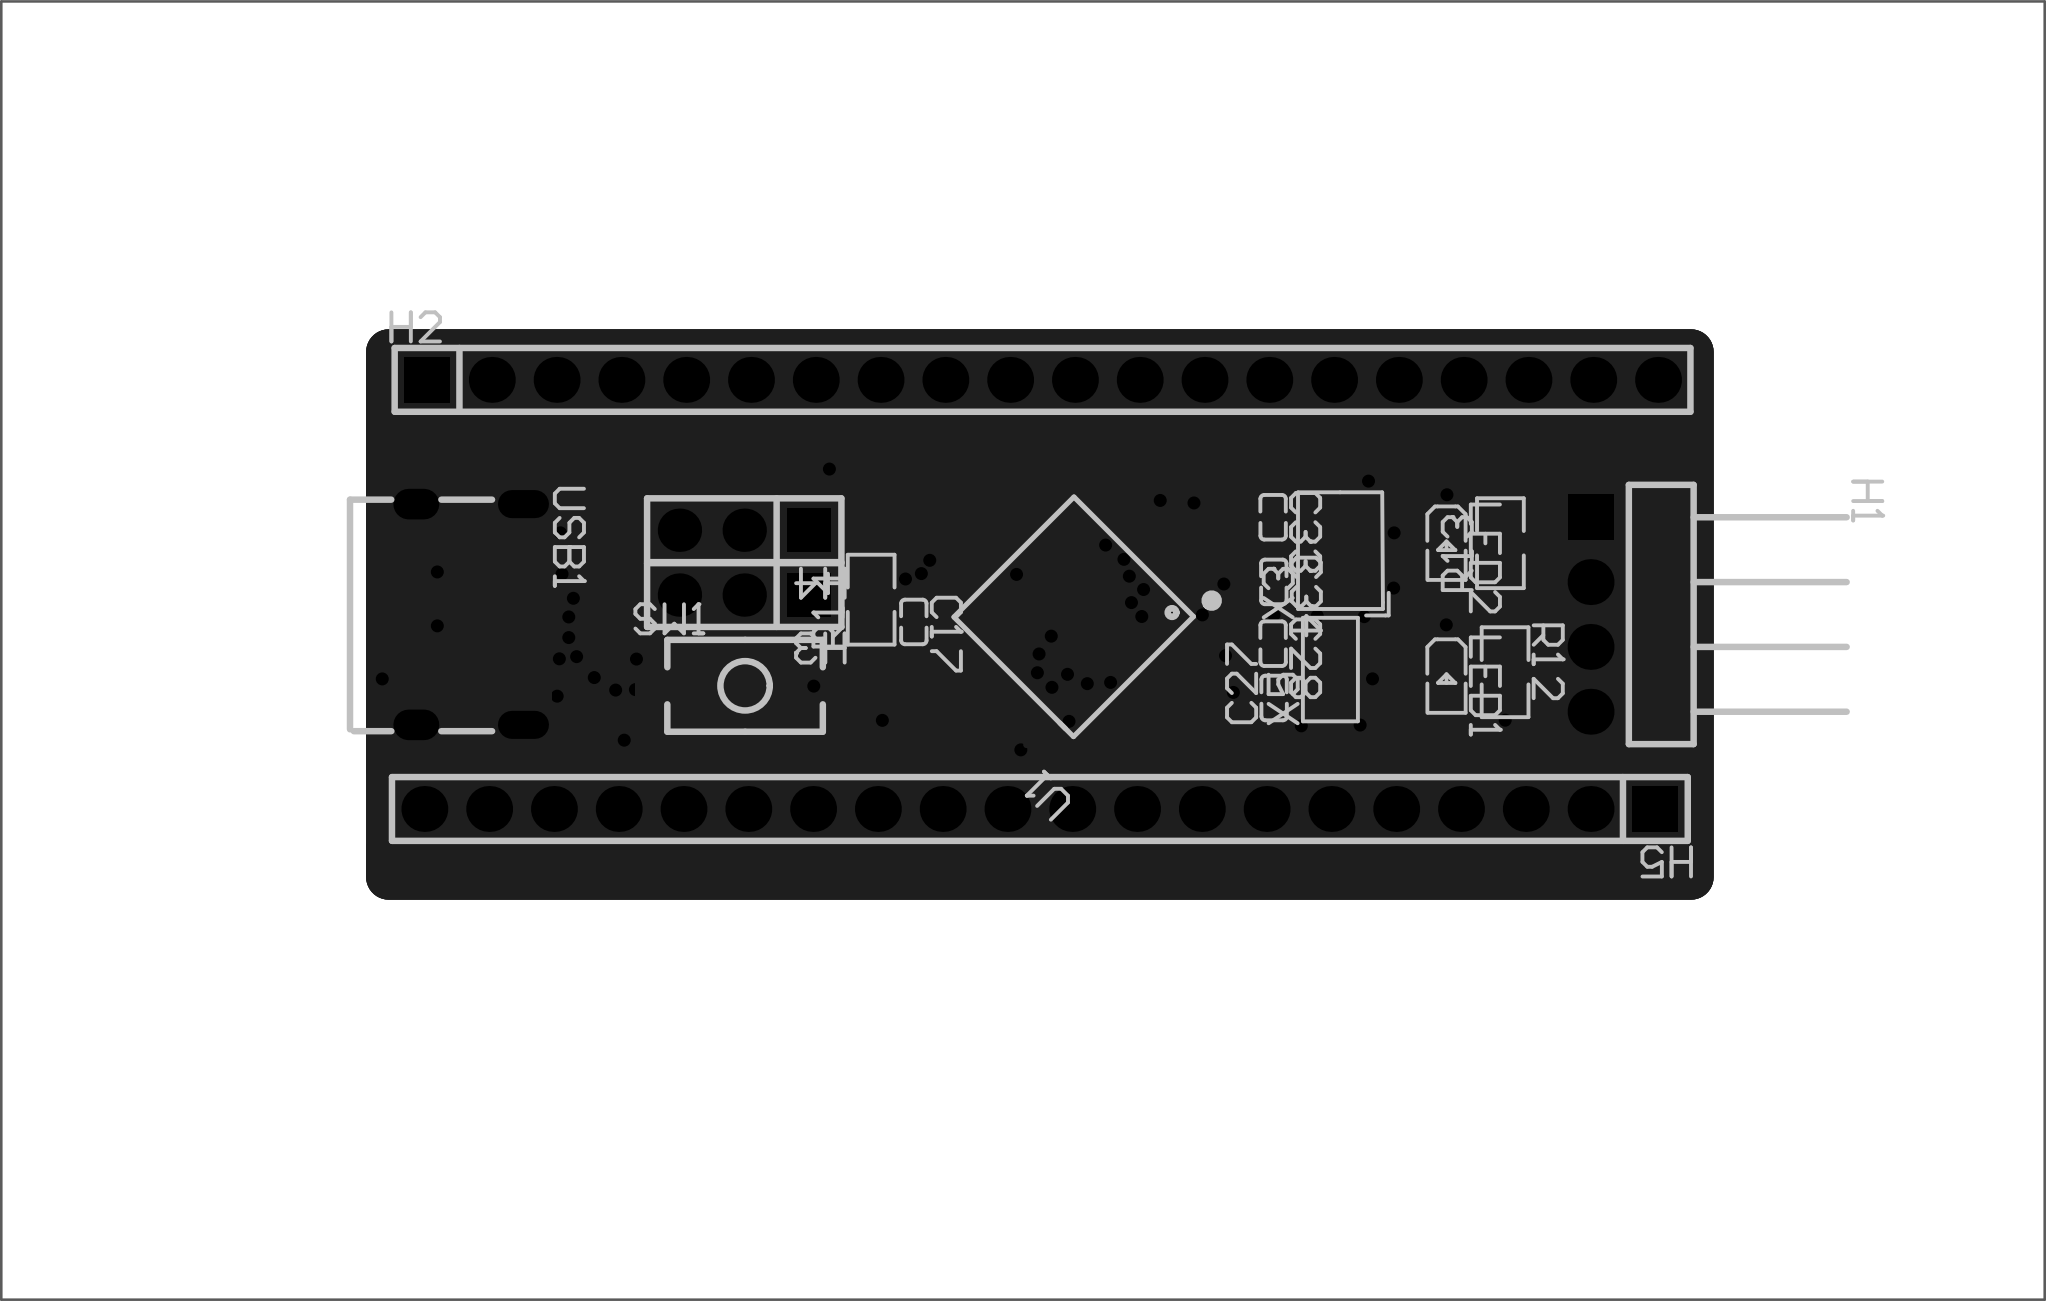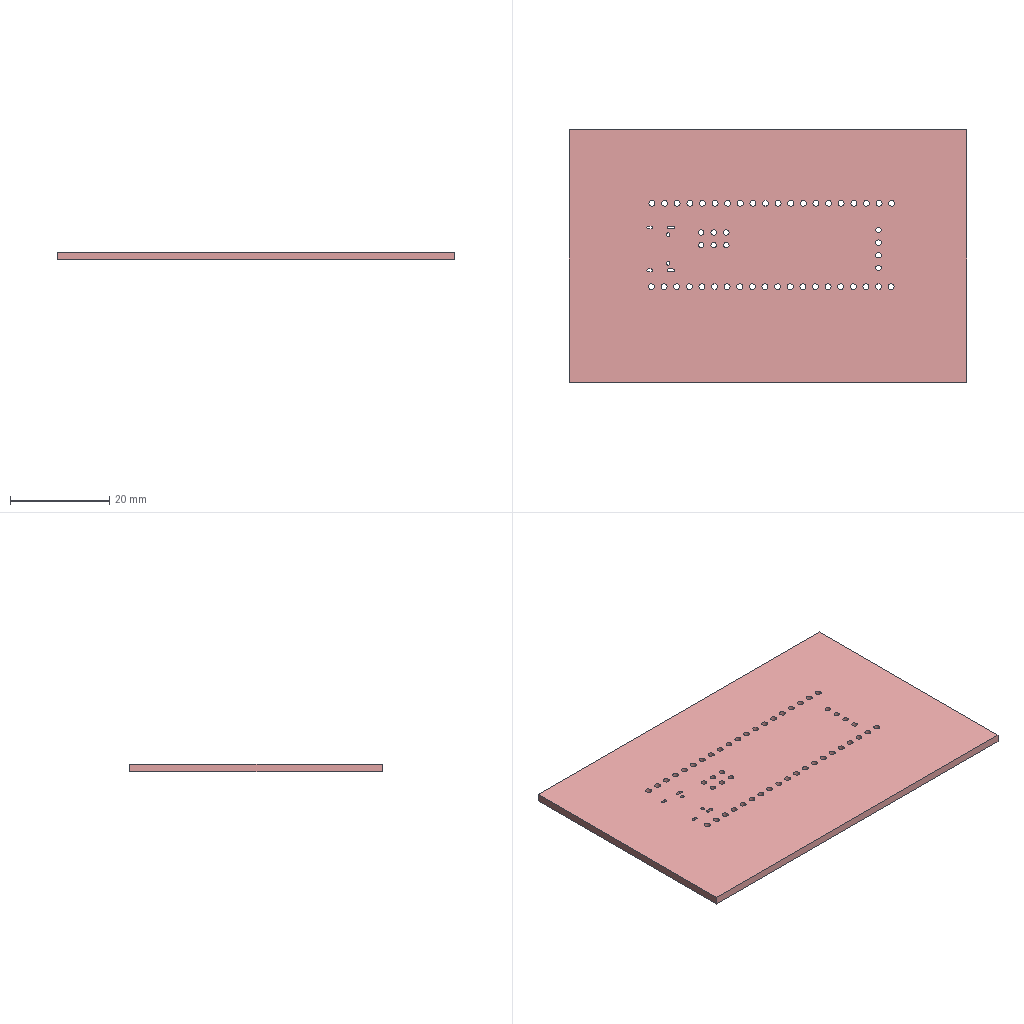Circuit board layout | Altium Designer | box 80.1 x 50.9 x 1.6 mm
Layer stack:
# Altium Designer layer stack of  (unit mm; dielectric type: 0 none, 1 core, 2 prepreg, 3 surface material)
index,name,kind,layer,copper_thickness_mm,dielectric_type,dielectric_thickness_mm,dielectric_material,dielectric_constant
0,Top Paste Mask Layer,other,,,,,,
1,Top Silkscreen Layer,other,,,,,,
2,Top Solder Mask Layer,dielectric,,,3,0.01,,3.3
3,Top Layer,copper,Top Layer,0.035,,,,
4,Dielectric1,dielectric,,,3,1.51,FR4,4.5
5,Bottom Layer,copper,Bottom Layer,0.035,,,,
6,Bottom Solder Mask Layer,dielectric,,,3,0.01,,3.3
7,Bottom Silkscreen Layer,other,,,,,,
8,Bottom Paste Mask Layer,other,,,,,,
# drill layer pairs: low layer,high layer
drill_pair,Top Layer,Bottom Layer
Part placement:
Designator,Comment,Layer,Footprint,Center-X(mm),Center-Y(mm),Rotation
C15,100nF,BottomLayer,C0402,96.879,92.261,270
C16,100nF,BottomLayer,C0402,103.205,92.261,270
C17,100nF,TopLayer,C0402,105.625,96.406,270
C18,100nF,BottomLayer,C0402,108.015,98.226,0
C19,100nF,BottomLayer,C0402,110.848,92.034,0
C20,100nF,BottomLayer,C0402,116.099,95.074,180
C21,100nF,BottomLayer,C0402,114.447,100.877,0
C22,100nF,BottomLayer,C0402,128.817,94.312,270
C23,1uF,BottomLayer,C0402,95.58,92.261,270
C24,1uF,BottomLayer,C0402,101.854,92.261,270
C27,12pF,TopLayer,C0402,119.749,93.425,90
C28,12pF,TopLayer,C0402,119.71,95.555,270
C33,12pF,TopLayer,C0402,119.71,100.508,270
C34,12pF,TopLayer,C0402,119.738,97.975,270
H1,DZ254W-11-04-65,TopLayer,HDR-TH_4P-P2.54-H-M-W10.3,132.156,96.698,270
H2,,TopLayer,HDR-TH_20P-P2.54-V-M-1,110.671,105.891,0
H3,,TopLayer,HDR-TH_3P-P2.54-V-M,98.976,97.46,180
H4,,TopLayer,HDR-TH_3P-P2.54-V-M,98.976,100,180
H5,,TopLayer,HDR-TH_20P-P2.54-V-M-1,110.566,89.078,180
LDO1,ME6211C33M5G-N,BottomLayer,SOT-23-5_L3.0-W1.7-P0.95-LS2.8-BL,99.306,92.464,90
LED1,NCD0603R1,TopLayer,LED0603-RD_RED,126.502,94.235,270
LED2,NCD0603B1,TopLayer,LED0603-RD,126.502,99.442,270
R9,5.1KΩ,BottomLayer,R0805,87.23,94.174,180
R10,5.1KΩ,BottomLayer,R0805,89.516,98.365,180
R11,1.5KΩ,BottomLayer,R0805,89.516,96.269,0
R12,1KΩ,TopLayer,R0805,128.804,94.436,270
R13,1KΩ,TopLayer,R0805,128.621,99.492,90
R14,10KΩ,TopLayer,R0805,103.952,97.278,90
R15,10KΩ,BottomLayer,R0805,98.494,101.879,0
R16,10KΩ,BottomLayer,R0805,94.624,101.915,0
SW1,TS-1101-B-W,TopLayer,KEY-SMD_2P-L6.0-W3.6-P7.4-LS8.0-L,99.009,93.904,0
U1,STM32F103C8T6,TopLayer,LQFP-48_L7.0-W7.0-P0.50-LS9.0-BL,111.894,96.626,135
USB1,TYPE-C 16PIN 2MD(073),TopLayer,USB-C-SMD_TYPE-C-6PIN-2MD-073,88.496,96.698,270
X3,8MHz,TopLayer,CRYSTAL-SMD_4P-L3.2-W2.5-BL-1,122.337,99.2,90
X5,32.768kHz,TopLayer,OSC-SMD_L3.2-W1.5,121.956,94.54,90
Pad and via stacks:
# Altium Designer via and pad stacks of  (unit mm). Each distinct definition once, with the count of objects using it.
# via: kind,start_layer,end_layer,hole_mm,diameter_mm,mode(0 simple;1 top-mid-bottom;2 full stack),diameter_per_layer,count,example_net
# pad: kind,layer,hole_mm,hole_type(0 round;1 square;2 slot),plating,top_size,top_shape(1 round;2 rect;3 octagon;9 rounded rect),mid_size,bottom_size,mode,footprint,size_per_layer,count,example
pad,Bottom Layer,0,0,plated,0.5x0.54,2,0.5x0.54,0.5x0.54,0,C0402,,18,C15.2
pad,Bottom Layer,0,0,plated,0.49x1.157,2,0.49x1.157,0.49x1.157,0,SOT-23-5_L3.0-W1.7-P0.95-LS2.8-BL,,3,LDO1.1
pad,Bottom Layer,0,0,plated,0.49x1.175,2,0.49x1.175,0.49x1.175,0,SOT-23-5_L3.0-W1.7-P0.95-LS2.8-BL,,2,LDO1.4
pad,Bottom Layer,0,0,plated,1.133x1.377,2,1.133x1.377,1.133x1.377,0,R0805,,10,R9.2
pad,Top Layer,0,0,plated,0.5x0.54,2,0.5x0.54,0.5x0.54,0,C0402,,10,C17.2
pad,Top Layer,0,0,plated,0.8x0.8,2,0.8x0.8,0.8x0.8,0,LED0603-RD_RED,,2,LED1.1
pad,Top Layer,0,0,plated,0.8x0.8,2,0.8x0.8,0.8x0.8,0,LED0603-RD,,2,LED2.2
pad,Top Layer,0,0,plated,1.133x1.377,2,1.133x1.377,1.133x1.377,0,R0805,,6,R12.2
pad,Top Layer,0,0,plated,1.2x1,2,1.2x1,1.2x1,0,KEY-SMD_2P-L6.0-W3.6-P7.4-LS8.0-L,,2,SW1.1
pad,Top Layer,0,0,plated,0.27x1.5,1,0.27x1.5,0.27x1.5,0,LQFP-48_L7.0-W7.0-P0.50-LS9.0-BL,,24,U1.1
pad,Top Layer,0,0,plated,1.5x0.27,1,1.5x0.27,1.5x0.27,0,LQFP-48_L7.0-W7.0-P0.50-LS9.0-BL,,24,U1.13
pad,Top Layer,0,0,plated,0.55x1.1,2,0.55x1.1,0.55x1.1,0,USB-C-SMD_TYPE-C-6PIN-2MD-073,,4,USB1.1
pad,Top Layer,0,0,plated,0.3x1.1,2,0.3x1.1,0.3x1.1,0,USB-C-SMD_TYPE-C-6PIN-2MD-073,,8,USB1.3
pad,Top Layer,0,0,plated,1.4x1.2,2,1.4x1.2,1.4x1.2,0,CRYSTAL-SMD_4P-L3.2-W2.5-BL-1,,4,X3.1
pad,Top Layer,0,0,plated,0.85x1.7,2,0.85x1.7,0.85x1.7,0,OSC-SMD_L3.2-W1.5,,2,X5.1
pad,Multi-Layer,1.1,0,plated,1.8x1.8,1,1.8x1.8,1.8x1.8,0,HDR-TH_4P-P2.54-H-M-W10.3,,3,H1.4
pad,Multi-Layer,1.1,0,plated,1.8x1.8,2,1.8x1.8,1.8x1.8,0,HDR-TH_4P-P2.54-H-M-W10.3,,1,H1.1
pad,Multi-Layer,1.2,0,plated,1.8x1.8,1,1.8x1.8,1.8x1.8,0,HDR-TH_20P-P2.54-V-M-1,,38,H2.20
pad,Multi-Layer,1.2,0,plated,1.8x1.8,2,1.8x1.8,1.8x1.8,0,HDR-TH_20P-P2.54-V-M-1,,2,H2.1
pad,Multi-Layer,1.1,0,plated,1.7x1.7,2,1.7x1.7,1.7x1.7,0,HDR-TH_3P-P2.54-V-M,,2,H3.1
pad,Multi-Layer,1.1,0,plated,1.7x1.7,1,1.7x1.7,1.7x1.7,0,HDR-TH_3P-P2.54-V-M,,4,H3.2
pad,Multi-Layer,0.6,2,plated,1.1x2,1,1.1x2,1.1x2,0,USB-C-SMD_TYPE-C-6PIN-2MD-073,,2,USB1.13
pad,Multi-Layer,0.6,2,plated,1.2x1.8,1,1.2x1.8,1.2x1.8,0,USB-C-SMD_TYPE-C-6PIN-2MD-073,,2,USB1.13
via,Top Layer,Bottom Layer,0.3048,0.508,0,,56,GND
Copper pours:
name,layer,net,type(0 solid;1 hatched;2 none)
Bottom Layer-+5V,Bottom Layer,+5V,0
Bottom Layer-3V3,Bottom Layer,3V3,0
Bottom Layer-3V3 1,Bottom Layer,3V3,0
Bottom Layer-3V3 2,Bottom Layer,3V3,0
Bottom Layer-GND,Bottom Layer,GND,0
Bottom Layer-GND 1,Bottom Layer,GND,0
Top Layer-GND,Top Layer,GND,0
Top Layer-GND 1,Top Layer,GND,0
Design rules, without the lines most boards share:
# Altium Designer design rules of  (exported by Altium Designer, unit mm)
# columns: name | kind | enabled | priority | scope1 | scope2 | descriptor | typed fields (field=value)
safeClearance1 | 0 | enabled | 2 | (InNet('USB_D-_PA11')) | (InNet('GND')) | Clearance Constraint (Gap=6mil) ((InNet('USB_D-_PA11'))),((InNet('GND'))) | gap=0.1524
safeClearance1_1 | 63 | enabled | 2 | All | All | Board Clearance Constraint (Gap=0mil) (All) |
copperThickness1oz | 0 | enabled | 3 | All | All | Clearance Constraint (Gap=5.984mil) (All),(All) | gap=0.152
copperThickness1oz_1 | 63 | enabled | 3 | All | All | Board Clearance Constraint (Gap=0mil) (All) |
PWR | 2 | enabled | 2 | (InNet('3V3') OR InNet('+5V') OR InNet('GND')) | All | Width Constraint (Min=5mil) (Max=100mil) (Preferred=15mil) ((InNet('3V3') OR InNet('+5V') OR InNet('GND'))) |
copperThickness1oz_2 | 2 | enabled | 3 | All | All | Width Constraint (Min=5mil) (Max=100mil) (Preferred=8mil) (All) |
differentialPair | 51 | enabled | 1 | All | All | Differential Pairs Uncoupled Length using the Gap Constraints (Min=4mil) (Max=5mil) (Prefered=5mil)  and Width Constraints (Min=5mil) (Max=100mil) (Prefered=9mil) (All) |
viaSize | 11 | enabled | 1 | All | All | Routing Via (MinHoleWidth=11.811mil) (MaxHoleWidth=248.031mil) (PreferredHoleWidth=12.008mil) (MinWidth=19.685mil) (MaxWidth=393.701mil) (PreferedWidth=20mil) (All) | via_min_hole=0.3 via_max_hole=6.3 via_preferred_diameter=0.508 via_preferred_hole=0.305
copperRegion_Top Layer | 20 | enabled | 1 | (OnLayer('Top Layer')) | All | Polygon Connect Rule(Direct Connect )(Conductor Width=10mil) (Relief Angle=90 Angle) (Entries=4) (Air Gap Width=10mil) ((OnLayer('Top Layer'))),(All) | connect_style(0=relief,1=direct,2=none)=1 relief_conductor_width=0.254 relief_entries=4
copperRegion_Bottom Layer | 20 | enabled | 2 | (OnLayer('Bottom Layer')) | All | Polygon Connect Rule(Direct Connect )(Conductor Width=10mil) (Relief Angle=90 Angle) (Entries=4) (Air Gap Width=10mil) ((OnLayer('Bottom Layer'))),(All) | connect_style(0=relief,1=direct,2=none)=1 relief_conductor_width=0.254 relief_entries=4
copperRegion | 20 | enabled | 3 | All | All | Polygon Connect Rule(Direct Connect )(Conductor Width=10mil) (Relief Angle=90 Angle) (Entries=4) (Air Gap Width=10mil) (All),(All) | connect_style(0=relief,1=direct,2=none)=1 relief_conductor_width=0.254 relief_entries=4